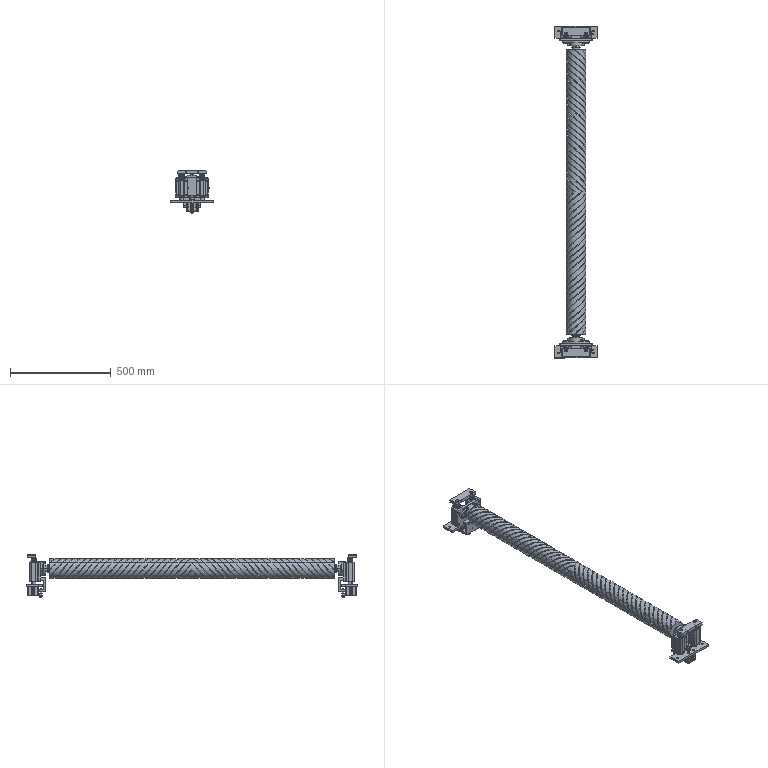Part | SolidWorks | features ReferencePattern 8, CompositeCurve 5, MirrorCompFeat 2 | 47 solids | 2130 faces | box 210 x 1644 x 211.13 mm | volume 12241603 mm3 | cylinder 1018 | plane 674 | cone 312 | spline 126 | commonest cylinder face diameters 96 x100 0.4 x92 5.2 x72 6.4 x68 11 x68 32 x48